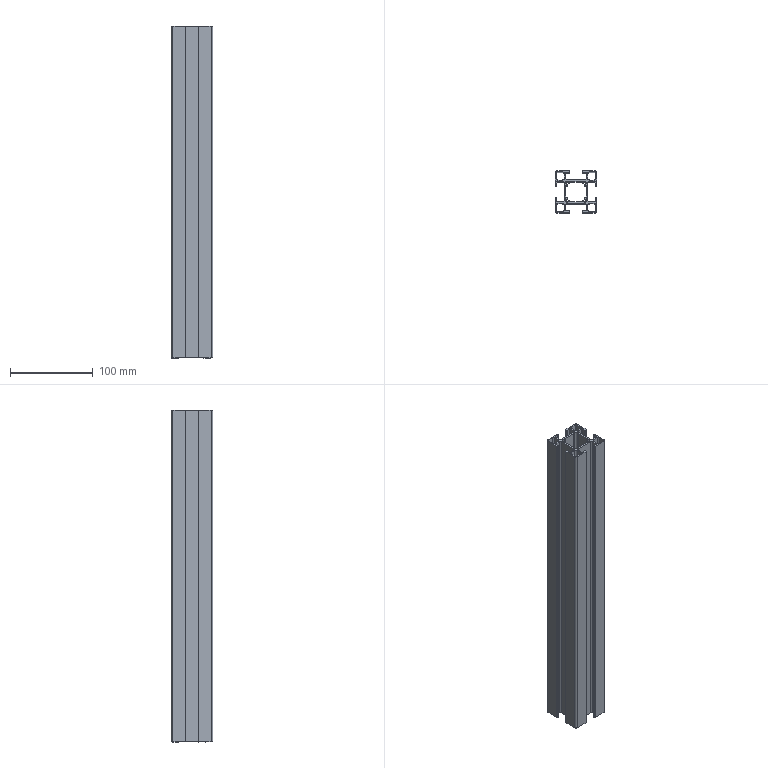Part | STEP file | 46A-00006CC11-400mm | 1 solid | 142 faces | box 50 x 50 x 400 mm | volume 234997 mm3 | cylinder 84 | plane 58 | commonest cylinder face diameters 1 x24 4 x24 1.5 x16 3.7 x8 6.7 x8 2 x4